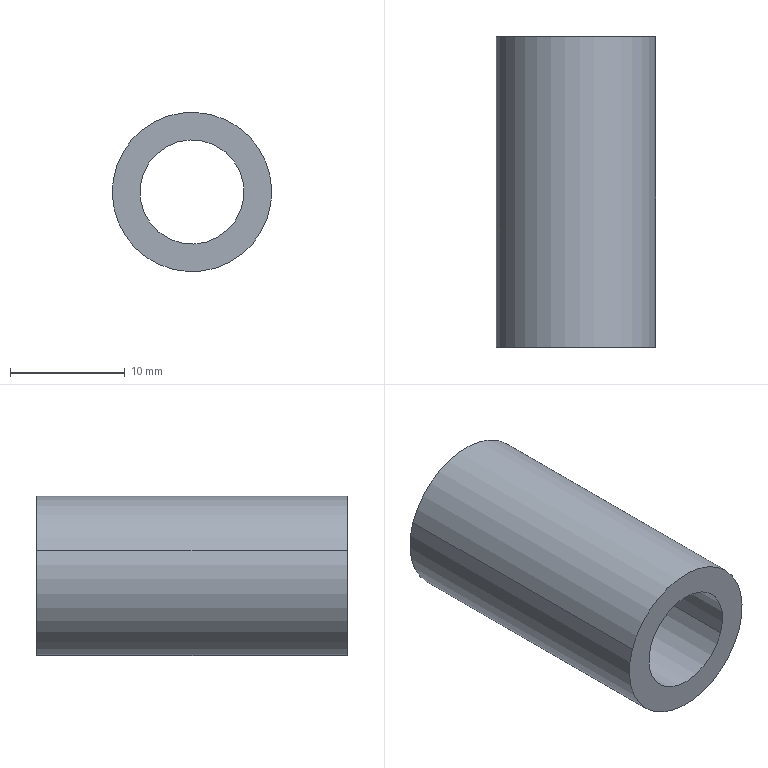Part | STEP file | 2026.6.15-Main Assembly图.sldasm-Part-187 | 1 solid | 6 faces | box 13.86 x 27 x 13.86 mm | volume 2333 mm3 | cylinder 4 | plane 2 | commonest cylinder face diameters 9.06 x2 13.86 x2
STEP:
#1=CARTESIAN_POINT('',(-1626.946,1437.764,3350.697));
#2=VERTEX_POINT('',#1);
#3=CARTESIAN_POINT('',(-1626.946,1410.764,3350.697));
#4=VERTEX_POINT('',#3);
#5=CARTESIAN_POINT('',(-1626.946,1410.764,3350.697));
#6=DIRECTION('',(0.,-1.,0.));
#7=VECTOR('',#6,1000.);
#8=LINE('',#5,#7);
#9=EDGE_CURVE('',#2,#4,#8,.T.);
#10=ORIENTED_EDGE('',*,*,#9,.T.);
#11=CARTESIAN_POINT('',(-1635.53,1410.764,3353.596));
#12=VERTEX_POINT('',#11);
#13=CARTESIAN_POINT('',(-1631.238,1410.764,3352.147));
#14=DIRECTION('',(0.,1.,0.));
#15=DIRECTION('',(-0.9474,0.,0.3199));
#16=AXIS2_PLACEMENT_3D('',#13,#14,#15);
#17=CIRCLE('',#16,4.53);
#18=EDGE_CURVE('',#12,#4,#17,.T.);
#19=ORIENTED_EDGE('',*,*,#18,.F.);
#20=CARTESIAN_POINT('',(-1635.53,1437.764,3353.596));
#21=VERTEX_POINT('',#20);
#22=CARTESIAN_POINT('',(-1635.53,1410.764,3353.596));
#23=DIRECTION('',(0.,-1.,0.));
#24=VECTOR('',#23,1000.);
#25=LINE('',#22,#24);
#26=EDGE_CURVE('',#21,#12,#25,.T.);
#27=ORIENTED_EDGE('',*,*,#26,.F.);
#28=CARTESIAN_POINT('',(-1631.238,1437.764,3352.147));
#29=DIRECTION('',(0.,1.,0.));
#30=DIRECTION('',(-0.9474,0.,0.3199));
#31=AXIS2_PLACEMENT_3D('',#28,#29,#30);
#32=CIRCLE('',#31,4.53);
#33=EDGE_CURVE('',#21,#2,#32,.T.);
#34=ORIENTED_EDGE('',*,*,#33,.T.);
#35=EDGE_LOOP('',(#10,#19,#27,#34));
#36=FACE_OUTER_BOUND('',#35,.T.);
#37=CARTESIAN_POINT('',(-1631.238,1410.764,3352.147));
#38=DIRECTION('',(0.,1.,0.));
#39=DIRECTION('',(0.9474,0.,-0.3199));
#40=AXIS2_PLACEMENT_3D('',#37,#38,#39);
#41=CYLINDRICAL_SURFACE('',#40,4.53);
#42=ADVANCED_FACE('',(#36),#41,.F.);
#43=CARTESIAN_POINT('',(-1637.804,1410.764,3354.364));
#44=VERTEX_POINT('',#43);
#45=CARTESIAN_POINT('',(-1624.673,1410.764,3349.93));
#46=VERTEX_POINT('',#45);
#47=CARTESIAN_POINT('',(-1631.238,1410.764,3352.147));
#48=DIRECTION('',(0.,1.,0.));
#49=DIRECTION('',(-0.9474,0.,0.3199));
#50=AXIS2_PLACEMENT_3D('',#47,#48,#49);
#51=CIRCLE('',#50,6.93);
#52=EDGE_CURVE('',#44,#46,#51,.T.);
#53=ORIENTED_EDGE('',*,*,#52,.F.);
#54=CARTESIAN_POINT('',(-1631.238,1410.764,3352.147));
#55=DIRECTION('',(0.,1.,0.));
#56=DIRECTION('',(-0.9474,0.,0.3199));
#57=AXIS2_PLACEMENT_3D('',#54,#55,#56);
#58=CIRCLE('',#57,6.93);
#59=EDGE_CURVE('',#46,#44,#58,.T.);
#60=ORIENTED_EDGE('',*,*,#59,.F.);
#61=EDGE_LOOP('',(#53,#60));
#62=FACE_OUTER_BOUND('',#61,.T.);
#63=ORIENTED_EDGE('',*,*,#18,.T.);
#64=CARTESIAN_POINT('',(-1631.238,1410.764,3352.147));
#65=DIRECTION('',(0.,1.,0.));
#66=DIRECTION('',(-0.9474,0.,0.3199));
#67=AXIS2_PLACEMENT_3D('',#64,#65,#66);
#68=CIRCLE('',#67,4.53);
#69=EDGE_CURVE('',#4,#12,#68,.T.);
#70=ORIENTED_EDGE('',*,*,#69,.T.);
#71=EDGE_LOOP('',(#63,#70));
#72=FACE_BOUND('',#71,.T.);
#73=CARTESIAN_POINT('',(-1631.238,1410.764,3352.147));
#74=DIRECTION('',(0.,-1.,0.));
#75=DIRECTION('',(0.,0.,-1.));
#76=AXIS2_PLACEMENT_3D('',#73,#74,#75);
#77=PLANE('',#76);
#78=ADVANCED_FACE('',(#62,#72),#77,.T.);
#79=CARTESIAN_POINT('',(-1637.804,1437.764,3354.364));
#80=VERTEX_POINT('',#79);
#81=CARTESIAN_POINT('',(-1624.673,1437.764,3349.93));
#82=VERTEX_POINT('',#81);
#83=CARTESIAN_POINT('',(-1631.238,1437.764,3352.147));
#84=DIRECTION('',(0.,-1.,0.));
#85=DIRECTION('',(-0.9474,0.,0.3199));
#86=AXIS2_PLACEMENT_3D('',#83,#84,#85);
#87=CIRCLE('',#86,6.93);
#88=EDGE_CURVE('',#80,#82,#87,.T.);
#89=ORIENTED_EDGE('',*,*,#88,.F.);
#90=CARTESIAN_POINT('',(-1631.238,1437.764,3352.147));
#91=DIRECTION('',(0.,-1.,0.));
#92=DIRECTION('',(-0.9474,0.,0.3199));
#93=AXIS2_PLACEMENT_3D('',#90,#91,#92);
#94=CIRCLE('',#93,6.93);
#95=EDGE_CURVE('',#82,#80,#94,.T.);
#96=ORIENTED_EDGE('',*,*,#95,.F.);
#97=EDGE_LOOP('',(#89,#96));
#98=FACE_OUTER_BOUND('',#97,.T.);
#99=ORIENTED_EDGE('',*,*,#33,.F.);
#100=CARTESIAN_POINT('',(-1631.238,1437.764,3352.147));
#101=DIRECTION('',(0.,1.,0.));
#102=DIRECTION('',(-0.9474,0.,0.3199));
#103=AXIS2_PLACEMENT_3D('',#100,#101,#102);
#104=CIRCLE('',#103,4.53);
#105=EDGE_CURVE('',#2,#21,#104,.T.);
#106=ORIENTED_EDGE('',*,*,#105,.F.);
#107=EDGE_LOOP('',(#99,#106));
#108=FACE_BOUND('',#107,.T.);
#109=CARTESIAN_POINT('',(-1631.238,1437.764,3352.147));
#110=DIRECTION('',(0.,-1.,0.));
#111=DIRECTION('',(0.,0.,-1.));
#112=AXIS2_PLACEMENT_3D('',#109,#110,#111);
#113=PLANE('',#112);
#114=ADVANCED_FACE('',(#98,#108),#113,.F.);
#115=CARTESIAN_POINT('',(-1624.673,1410.764,3349.93));
#116=DIRECTION('',(0.,-1.,0.));
#117=VECTOR('',#116,1000.);
#118=LINE('',#115,#117);
#119=EDGE_CURVE('',#82,#46,#118,.T.);
#120=ORIENTED_EDGE('',*,*,#119,.T.);
#121=ORIENTED_EDGE('',*,*,#59,.T.);
#122=CARTESIAN_POINT('',(-1637.804,1410.764,3354.364));
#123=DIRECTION('',(0.,-1.,0.));
#124=VECTOR('',#123,1000.);
#125=LINE('',#122,#124);
#126=EDGE_CURVE('',#80,#44,#125,.T.);
#127=ORIENTED_EDGE('',*,*,#126,.F.);
#128=ORIENTED_EDGE('',*,*,#88,.T.);
#129=EDGE_LOOP('',(#120,#121,#127,#128));
#130=FACE_OUTER_BOUND('',#129,.T.);
#131=CARTESIAN_POINT('',(-1631.238,1410.764,3352.147));
#132=DIRECTION('',(0.,1.,0.));
#133=DIRECTION('',(0.9474,0.,-0.3199));
#134=AXIS2_PLACEMENT_3D('',#131,#132,#133);
#135=CYLINDRICAL_SURFACE('',#134,6.93);
#136=ADVANCED_FACE('',(#130),#135,.T.);
#137=ORIENTED_EDGE('',*,*,#69,.F.);
#138=ORIENTED_EDGE('',*,*,#9,.F.);
#139=ORIENTED_EDGE('',*,*,#105,.T.);
#140=ORIENTED_EDGE('',*,*,#26,.T.);
#141=EDGE_LOOP('',(#137,#138,#139,#140));
#142=FACE_OUTER_BOUND('',#141,.T.);
#143=CARTESIAN_POINT('',(-1631.238,1410.764,3352.147));
#144=DIRECTION('',(0.,1.,0.));
#145=DIRECTION('',(0.9474,0.,-0.3199));
#146=AXIS2_PLACEMENT_3D('',#143,#144,#145);
#147=CYLINDRICAL_SURFACE('',#146,4.53);
#148=ADVANCED_FACE('',(#142),#147,.F.);
#149=ORIENTED_EDGE('',*,*,#52,.T.);
#150=ORIENTED_EDGE('',*,*,#119,.F.);
#151=ORIENTED_EDGE('',*,*,#95,.T.);
#152=ORIENTED_EDGE('',*,*,#126,.T.);
#153=EDGE_LOOP('',(#149,#150,#151,#152));
#154=FACE_OUTER_BOUND('',#153,.T.);
#155=CARTESIAN_POINT('',(-1631.238,1410.764,3352.147));
#156=DIRECTION('',(0.,1.,0.));
#157=DIRECTION('',(0.9474,0.,-0.3199));
#158=AXIS2_PLACEMENT_3D('',#155,#156,#157);
#159=CYLINDRICAL_SURFACE('',#158,6.93);
#160=ADVANCED_FACE('',(#154),#159,.T.);
#161=CLOSED_SHELL('',(#42,#78,#114,#136,#148,#160));
#162=MANIFOLD_SOLID_BREP('',#161);
#163=CARTESIAN_POINT('',(0.,0.,0.));
#164=DIRECTION('',(0.,0.,1.));
#165=DIRECTION('',(1.,0.,0.));
#166=AXIS2_PLACEMENT_3D('',#163,#164,#165);
#167=(LENGTH_UNIT()NAMED_UNIT(*)SI_UNIT(.MILLI.,.METRE.));
#168=UNCERTAINTY_MEASURE_WITH_UNIT(LENGTH_MEASURE(0.00001),#167,'','');
#169=(NAMED_UNIT(*)PLANE_ANGLE_UNIT()SI_UNIT($,.RADIAN.));
#170=(NAMED_UNIT(*)SI_UNIT($,.STERADIAN.)SOLID_ANGLE_UNIT());
#171=(GEOMETRIC_REPRESENTATION_CONTEXT(3)GLOBAL_UNCERTAINTY_ASSIGNED_CONTEXT((#168))GLOBAL_UNIT_ASSIGNED_CONTEXT((#167,#169,#170))REPRESENTATION_CONTEXT('',''));
#172=ADVANCED_BREP_SHAPE_REPRESENTATION('',(#162,#166),#171);